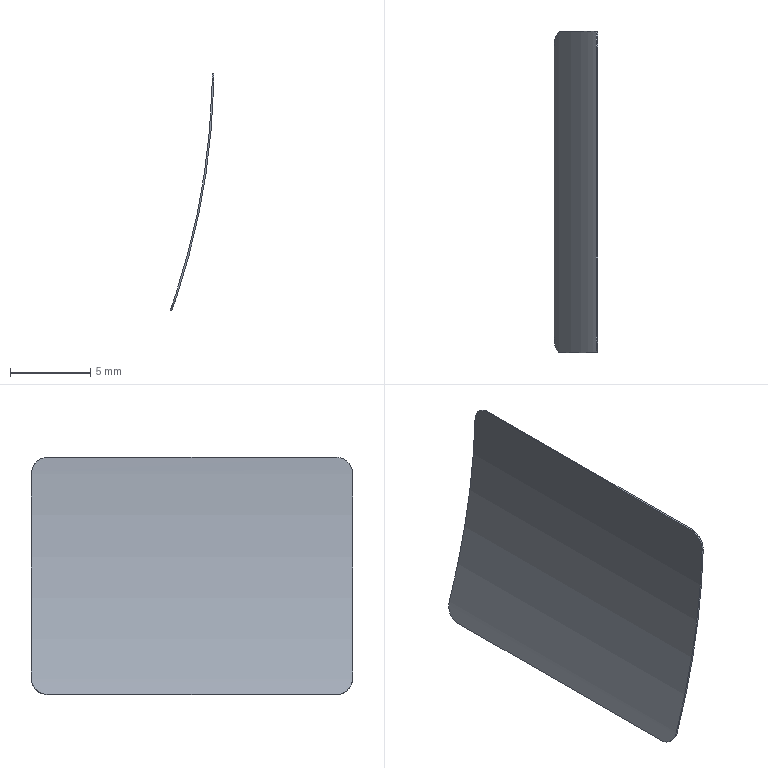Part | SolidWorks | features BaseBody 1 | 1 solid | 10 faces | box 2.721 x 20 x 14.787 mm | volume 30.051 mm3 | cylinder 6 | plane 4 | commonest cylinder face diameters 2 x4 90.8 x1 91 x1
STEP:
#1=CARTESIAN_POINT('',(2075.604,-17.405,824.629));
#2=VERTEX_POINT('',#1);
#3=CARTESIAN_POINT('',(2077.876,-17.405,837.429));
#4=VERTEX_POINT('',#3);
#5=CARTESIAN_POINT('',(2032.4,-17.405,838.898));
#6=DIRECTION('',(0.,-1.,0.));
#7=DIRECTION('',(0.9496,0.,-0.3136));
#8=AXIS2_PLACEMENT_3D('',#5,#6,#7);
#9=CIRCLE('',#8,45.5);
#10=EDGE_CURVE('',#2,#4,#9,.T.);
#11=ORIENTED_EDGE('',*,*,#10,.F.);
#12=CARTESIAN_POINT('',(2075.505,-17.405,824.646));
#13=VERTEX_POINT('',#12);
#14=CARTESIAN_POINT('',(2075.604,-17.405,824.629));
#15=DIRECTION('',(-0.9846,0.,0.1747));
#16=VECTOR('',#15,1000.);
#17=LINE('',#14,#16);
#18=EDGE_CURVE('',#2,#13,#17,.T.);
#19=ORIENTED_EDGE('',*,*,#18,.T.);
#20=CARTESIAN_POINT('',(2077.776,-17.405,837.446));
#21=VERTEX_POINT('',#20);
#22=CARTESIAN_POINT('',(2032.4,-17.405,838.898));
#23=DIRECTION('',(0.,1.,0.));
#24=DIRECTION('',(0.9995,0.,-0.03198));
#25=AXIS2_PLACEMENT_3D('',#22,#23,#24);
#26=CIRCLE('',#25,45.4);
#27=EDGE_CURVE('',#21,#13,#26,.T.);
#28=ORIENTED_EDGE('',*,*,#27,.F.);
#29=CARTESIAN_POINT('',(2077.776,-17.405,837.446));
#30=DIRECTION('',(0.9846,0.,-0.1747));
#31=VECTOR('',#30,1000.);
#32=LINE('',#29,#31);
#33=EDGE_CURVE('',#21,#4,#32,.T.);
#34=ORIENTED_EDGE('',*,*,#33,.T.);
#35=EDGE_LOOP('',(#11,#19,#28,#34));
#36=FACE_OUTER_BOUND('',#35,.T.);
#37=CARTESIAN_POINT('',(2032.4,-17.405,838.898));
#38=DIRECTION('',(0.,-1.,0.));
#39=DIRECTION('',(-0.1747,0.,-0.9846));
#40=AXIS2_PLACEMENT_3D('',#37,#38,#39);
#41=PLANE('',#40);
#42=ADVANCED_FACE('',(#36),#41,.F.);
#43=CARTESIAN_POINT('',(2077.897,-18.405,838.44));
#44=VERTEX_POINT('',#43);
#45=CARTESIAN_POINT('',(2077.876,-17.405,837.429));
#46=CARTESIAN_POINT('',(2077.88,-17.405,837.561));
#47=CARTESIAN_POINT('',(2077.884,-17.431,837.692));
#48=CARTESIAN_POINT('',(2077.89,-17.53,837.936));
#49=CARTESIAN_POINT('',(2077.892,-17.604,838.048));
#50=CARTESIAN_POINT('',(2077.896,-17.88,838.329));
#51=CARTESIAN_POINT('',(2077.897,-18.139,838.44));
#52=CARTESIAN_POINT('',(2077.897,-18.405,838.44));
#53=B_SPLINE_CURVE_WITH_KNOTS('',3,(#45,#46,#47,#48,#49,#50,#51,#52),.UNSPECIFIED.,.F.,.F.,(4,2,2,4),(0.,0.0003928,0.0007857,0.001571),.UNSPECIFIED.);
#54=EDGE_CURVE('',#4,#44,#53,.T.);
#55=ORIENTED_EDGE('',*,*,#54,.F.);
#56=ORIENTED_EDGE('',*,*,#33,.F.);
#57=CARTESIAN_POINT('',(2077.797,-18.405,838.458));
#58=VERTEX_POINT('',#57);
#59=CARTESIAN_POINT('',(2077.797,-18.405,838.458));
#60=CARTESIAN_POINT('',(2077.797,-18.272,838.458));
#61=CARTESIAN_POINT('',(2077.797,-18.142,838.431));
#62=CARTESIAN_POINT('',(2077.796,-17.899,838.329));
#63=CARTESIAN_POINT('',(2077.795,-17.788,838.253));
#64=CARTESIAN_POINT('',(2077.792,-17.604,838.066));
#65=CARTESIAN_POINT('',(2077.79,-17.53,837.953));
#66=CARTESIAN_POINT('',(2077.784,-17.431,837.711));
#67=CARTESIAN_POINT('',(2077.781,-17.405,837.579));
#68=CARTESIAN_POINT('',(2077.776,-17.405,837.446));
#69=B_SPLINE_CURVE_WITH_KNOTS('',3,(#59,#60,#61,#62,#63,#64,#65,#66,#67,#68),.UNSPECIFIED.,.F.,.F.,(4,2,2,2,4),(0.,0.0003929,0.0007857,0.001179,0.001571),.UNSPECIFIED.);
#70=EDGE_CURVE('',#58,#21,#69,.T.);
#71=ORIENTED_EDGE('',*,*,#70,.F.);
#72=CARTESIAN_POINT('',(2077.797,-18.405,838.458));
#73=DIRECTION('',(0.9846,0.,-0.1747));
#74=VECTOR('',#73,1000.);
#75=LINE('',#72,#74);
#76=EDGE_CURVE('',#58,#44,#75,.T.);
#77=ORIENTED_EDGE('',*,*,#76,.T.);
#78=EDGE_LOOP('',(#55,#56,#71,#77));
#79=FACE_OUTER_BOUND('',#78,.T.);
#80=CARTESIAN_POINT('',(2077.583,-18.405,837.481));
#81=DIRECTION('',(0.9846,0.,-0.1747));
#82=DIRECTION('',(0.,-1.,0.));
#83=AXIS2_PLACEMENT_3D('',#80,#81,#82);
#84=CYLINDRICAL_SURFACE('',#83,1.);
#85=ADVANCED_FACE('',(#79),#84,.T.);
#86=CARTESIAN_POINT('',(2077.797,-36.405,838.458));
#87=VERTEX_POINT('',#86);
#88=CARTESIAN_POINT('',(2077.797,-18.405,838.458));
#89=DIRECTION('',(0.,-1.,0.));
#90=VECTOR('',#89,1000.);
#91=LINE('',#88,#90);
#92=EDGE_CURVE('',#58,#87,#91,.T.);
#93=ORIENTED_EDGE('',*,*,#92,.T.);
#94=CARTESIAN_POINT('',(2077.897,-36.405,838.44));
#95=VERTEX_POINT('',#94);
#96=CARTESIAN_POINT('',(2077.897,-36.405,838.44));
#97=DIRECTION('',(-0.9846,0.,0.1747));
#98=VECTOR('',#97,1000.);
#99=LINE('',#96,#98);
#100=EDGE_CURVE('',#95,#87,#99,.T.);
#101=ORIENTED_EDGE('',*,*,#100,.F.);
#102=CARTESIAN_POINT('',(2077.897,-18.405,838.44));
#103=DIRECTION('',(0.,-1.,0.));
#104=VECTOR('',#103,1000.);
#105=LINE('',#102,#104);
#106=EDGE_CURVE('',#44,#95,#105,.T.);
#107=ORIENTED_EDGE('',*,*,#106,.F.);
#108=ORIENTED_EDGE('',*,*,#76,.F.);
#109=EDGE_LOOP('',(#93,#101,#107,#108));
#110=FACE_OUTER_BOUND('',#109,.T.);
#111=CARTESIAN_POINT('',(2077.897,-17.405,838.44));
#112=DIRECTION('',(0.1747,0.,0.9846));
#113=DIRECTION('',(0.9846,0.,-0.1747));
#114=AXIS2_PLACEMENT_3D('',#111,#112,#113);
#115=PLANE('',#114);
#116=ADVANCED_FACE('',(#110),#115,.T.);
#117=ORIENTED_EDGE('',*,*,#106,.T.);
#118=CARTESIAN_POINT('',(2077.876,-37.405,837.429));
#119=VERTEX_POINT('',#118);
#120=CARTESIAN_POINT('',(2077.897,-36.405,838.44));
#121=CARTESIAN_POINT('',(2077.897,-36.538,838.44));
#122=CARTESIAN_POINT('',(2077.897,-36.668,838.414));
#123=CARTESIAN_POINT('',(2077.896,-36.911,838.311));
#124=CARTESIAN_POINT('',(2077.895,-37.022,838.236));
#125=CARTESIAN_POINT('',(2077.892,-37.206,838.049));
#126=CARTESIAN_POINT('',(2077.89,-37.28,837.936));
#127=CARTESIAN_POINT('',(2077.884,-37.379,837.693));
#128=CARTESIAN_POINT('',(2077.88,-37.405,837.561));
#129=CARTESIAN_POINT('',(2077.876,-37.405,837.429));
#130=B_SPLINE_CURVE_WITH_KNOTS('',3,(#120,#121,#122,#123,#124,#125,#126,#127,#128,#129),.UNSPECIFIED.,.F.,.F.,(4,2,2,2,4),(0.,0.0003928,0.0007857,0.001179,0.001571),.UNSPECIFIED.);
#131=EDGE_CURVE('',#95,#119,#130,.T.);
#132=ORIENTED_EDGE('',*,*,#131,.T.);
#133=CARTESIAN_POINT('',(2075.604,-37.405,824.629));
#134=VERTEX_POINT('',#133);
#135=CARTESIAN_POINT('',(2032.4,-37.405,838.898));
#136=DIRECTION('',(0.,-1.,0.));
#137=DIRECTION('',(0.9496,0.,-0.3136));
#138=AXIS2_PLACEMENT_3D('',#135,#136,#137);
#139=CIRCLE('',#138,45.5);
#140=EDGE_CURVE('',#134,#119,#139,.T.);
#141=ORIENTED_EDGE('',*,*,#140,.F.);
#142=CARTESIAN_POINT('',(2075.276,-36.405,823.671));
#143=VERTEX_POINT('',#142);
#144=CARTESIAN_POINT('',(2075.604,-37.405,824.629));
#145=CARTESIAN_POINT('',(2075.562,-37.405,824.503));
#146=CARTESIAN_POINT('',(2075.521,-37.379,824.379));
#147=CARTESIAN_POINT('',(2075.442,-37.28,824.148));
#148=CARTESIAN_POINT('',(2075.406,-37.206,824.042));
#149=CARTESIAN_POINT('',(2075.314,-36.93,823.776));
#150=CARTESIAN_POINT('',(2075.276,-36.671,823.671));
#151=CARTESIAN_POINT('',(2075.276,-36.405,823.671));
#152=B_SPLINE_CURVE_WITH_KNOTS('',3,(#144,#145,#146,#147,#148,#149,#150,#151),.UNSPECIFIED.,.F.,.F.,(4,2,2,4),(0.,0.0003928,0.0007857,0.001571),.UNSPECIFIED.);
#153=EDGE_CURVE('',#134,#143,#152,.T.);
#154=ORIENTED_EDGE('',*,*,#153,.T.);
#155=CARTESIAN_POINT('',(2075.276,-18.405,823.671));
#156=VERTEX_POINT('',#155);
#157=CARTESIAN_POINT('',(2075.276,-18.405,823.671));
#158=DIRECTION('',(0.,-1.,0.));
#159=VECTOR('',#158,1000.);
#160=LINE('',#157,#159);
#161=EDGE_CURVE('',#156,#143,#160,.T.);
#162=ORIENTED_EDGE('',*,*,#161,.F.);
#163=CARTESIAN_POINT('',(2075.276,-18.405,823.671));
#164=CARTESIAN_POINT('',(2075.276,-18.272,823.671));
#165=CARTESIAN_POINT('',(2075.285,-18.142,823.696));
#166=CARTESIAN_POINT('',(2075.319,-17.899,823.793));
#167=CARTESIAN_POINT('',(2075.344,-17.788,823.865));
#168=CARTESIAN_POINT('',(2075.406,-17.604,824.041));
#169=CARTESIAN_POINT('',(2075.442,-17.53,824.148));
#170=CARTESIAN_POINT('',(2075.52,-17.431,824.377));
#171=CARTESIAN_POINT('',(2075.562,-17.405,824.503));
#172=CARTESIAN_POINT('',(2075.604,-17.405,824.629));
#173=B_SPLINE_CURVE_WITH_KNOTS('',3,(#163,#164,#165,#166,#167,#168,#169,#170,#171,#172),.UNSPECIFIED.,.F.,.F.,(4,2,2,2,4),(0.,0.0003928,0.0007857,0.001179,0.001571),.UNSPECIFIED.);
#174=EDGE_CURVE('',#156,#2,#173,.T.);
#175=ORIENTED_EDGE('',*,*,#174,.T.);
#176=ORIENTED_EDGE('',*,*,#10,.T.);
#177=ORIENTED_EDGE('',*,*,#54,.T.);
#178=EDGE_LOOP('',(#117,#132,#141,#154,#162,#175,#176,#177));
#179=FACE_OUTER_BOUND('',#178,.T.);
#180=CARTESIAN_POINT('',(2032.4,-17.405,838.898));
#181=DIRECTION('',(0.,-1.,0.));
#182=DIRECTION('',(-0.1747,0.,-0.9846));
#183=AXIS2_PLACEMENT_3D('',#180,#181,#182);
#184=CYLINDRICAL_SURFACE('',#183,45.5);
#185=ADVANCED_FACE('',(#179),#184,.T.);
#186=CARTESIAN_POINT('',(2075.176,-18.405,823.689));
#187=VERTEX_POINT('',#186);
#188=CARTESIAN_POINT('',(2075.505,-17.405,824.646));
#189=CARTESIAN_POINT('',(2075.463,-17.405,824.52));
#190=CARTESIAN_POINT('',(2075.421,-17.431,824.397));
#191=CARTESIAN_POINT('',(2075.343,-17.53,824.165));
#192=CARTESIAN_POINT('',(2075.306,-17.604,824.06));
#193=CARTESIAN_POINT('',(2075.214,-17.88,823.794));
#194=CARTESIAN_POINT('',(2075.176,-18.139,823.689));
#195=CARTESIAN_POINT('',(2075.176,-18.405,823.689));
#196=B_SPLINE_CURVE_WITH_KNOTS('',3,(#188,#189,#190,#191,#192,#193,#194,#195),.UNSPECIFIED.,.F.,.F.,(4,2,2,4),(0.,0.0003929,0.0007857,0.001571),.UNSPECIFIED.);
#197=EDGE_CURVE('',#13,#187,#196,.T.);
#198=ORIENTED_EDGE('',*,*,#197,.F.);
#199=ORIENTED_EDGE('',*,*,#18,.F.);
#200=ORIENTED_EDGE('',*,*,#174,.F.);
#201=CARTESIAN_POINT('',(2075.276,-18.405,823.671));
#202=DIRECTION('',(-0.9846,0.,0.1747));
#203=VECTOR('',#202,1000.);
#204=LINE('',#201,#203);
#205=EDGE_CURVE('',#156,#187,#204,.T.);
#206=ORIENTED_EDGE('',*,*,#205,.T.);
#207=EDGE_LOOP('',(#198,#199,#200,#206));
#208=FACE_OUTER_BOUND('',#207,.T.);
#209=CARTESIAN_POINT('',(2076.105,-18.405,824.54));
#210=DIRECTION('',(-0.9846,0.,0.1747));
#211=DIRECTION('',(0.,-1.,0.));
#212=AXIS2_PLACEMENT_3D('',#209,#210,#211);
#213=CYLINDRICAL_SURFACE('',#212,1.);
#214=ADVANCED_FACE('',(#208),#213,.T.);
#215=ORIENTED_EDGE('',*,*,#161,.T.);
#216=CARTESIAN_POINT('',(2075.176,-36.405,823.689));
#217=VERTEX_POINT('',#216);
#218=CARTESIAN_POINT('',(2075.176,-36.405,823.689));
#219=DIRECTION('',(0.9846,0.,-0.1747));
#220=VECTOR('',#219,1000.);
#221=LINE('',#218,#220);
#222=EDGE_CURVE('',#217,#143,#221,.T.);
#223=ORIENTED_EDGE('',*,*,#222,.F.);
#224=CARTESIAN_POINT('',(2075.176,-18.405,823.689));
#225=DIRECTION('',(0.,-1.,0.));
#226=VECTOR('',#225,1000.);
#227=LINE('',#224,#226);
#228=EDGE_CURVE('',#187,#217,#227,.T.);
#229=ORIENTED_EDGE('',*,*,#228,.F.);
#230=ORIENTED_EDGE('',*,*,#205,.F.);
#231=EDGE_LOOP('',(#215,#223,#229,#230));
#232=FACE_OUTER_BOUND('',#231,.T.);
#233=CARTESIAN_POINT('',(2075.176,-17.405,823.689));
#234=DIRECTION('',(-0.1747,0.,-0.9846));
#235=DIRECTION('',(-0.9846,0.,0.1747));
#236=AXIS2_PLACEMENT_3D('',#233,#234,#235);
#237=PLANE('',#236);
#238=ADVANCED_FACE('',(#232),#237,.T.);
#239=ORIENTED_EDGE('',*,*,#27,.T.);
#240=ORIENTED_EDGE('',*,*,#197,.T.);
#241=ORIENTED_EDGE('',*,*,#228,.T.);
#242=CARTESIAN_POINT('',(2075.505,-37.405,824.646));
#243=VERTEX_POINT('',#242);
#244=CARTESIAN_POINT('',(2075.176,-36.405,823.689));
#245=CARTESIAN_POINT('',(2075.176,-36.538,823.689));
#246=CARTESIAN_POINT('',(2075.185,-36.668,823.714));
#247=CARTESIAN_POINT('',(2075.219,-36.911,823.811));
#248=CARTESIAN_POINT('',(2075.245,-37.022,823.882));
#249=CARTESIAN_POINT('',(2075.306,-37.206,824.059));
#250=CARTESIAN_POINT('',(2075.343,-37.28,824.166));
#251=CARTESIAN_POINT('',(2075.421,-37.379,824.395));
#252=CARTESIAN_POINT('',(2075.463,-37.405,824.52));
#253=CARTESIAN_POINT('',(2075.505,-37.405,824.646));
#254=B_SPLINE_CURVE_WITH_KNOTS('',3,(#244,#245,#246,#247,#248,#249,#250,#251,#252,#253),.UNSPECIFIED.,.F.,.F.,(4,2,2,2,4),(0.,0.0003929,0.0007857,0.001179,0.001571),.UNSPECIFIED.);
#255=EDGE_CURVE('',#217,#243,#254,.T.);
#256=ORIENTED_EDGE('',*,*,#255,.T.);
#257=CARTESIAN_POINT('',(2077.776,-37.405,837.446));
#258=VERTEX_POINT('',#257);
#259=CARTESIAN_POINT('',(2032.4,-37.405,838.898));
#260=DIRECTION('',(0.,1.,0.));
#261=DIRECTION('',(0.9995,0.,-0.03198));
#262=AXIS2_PLACEMENT_3D('',#259,#260,#261);
#263=CIRCLE('',#262,45.4);
#264=EDGE_CURVE('',#258,#243,#263,.T.);
#265=ORIENTED_EDGE('',*,*,#264,.F.);
#266=CARTESIAN_POINT('',(2077.776,-37.405,837.446));
#267=CARTESIAN_POINT('',(2077.781,-37.405,837.579));
#268=CARTESIAN_POINT('',(2077.784,-37.379,837.709));
#269=CARTESIAN_POINT('',(2077.79,-37.28,837.954));
#270=CARTESIAN_POINT('',(2077.792,-37.206,838.066));
#271=CARTESIAN_POINT('',(2077.797,-36.93,838.347));
#272=CARTESIAN_POINT('',(2077.797,-36.671,838.458));
#273=CARTESIAN_POINT('',(2077.797,-36.405,838.458));
#274=B_SPLINE_CURVE_WITH_KNOTS('',3,(#266,#267,#268,#269,#270,#271,#272,#273),.UNSPECIFIED.,.F.,.F.,(4,2,2,4),(0.,0.0003929,0.0007857,0.001571),.UNSPECIFIED.);
#275=EDGE_CURVE('',#258,#87,#274,.T.);
#276=ORIENTED_EDGE('',*,*,#275,.T.);
#277=ORIENTED_EDGE('',*,*,#92,.F.);
#278=ORIENTED_EDGE('',*,*,#70,.T.);
#279=EDGE_LOOP('',(#239,#240,#241,#256,#265,#276,#277,#278));
#280=FACE_OUTER_BOUND('',#279,.T.);
#281=CARTESIAN_POINT('',(2032.4,-17.405,838.898));
#282=DIRECTION('',(0.,-1.,0.));
#283=DIRECTION('',(-0.1747,0.,-0.9846));
#284=AXIS2_PLACEMENT_3D('',#281,#282,#283);
#285=CYLINDRICAL_SURFACE('',#284,45.4);
#286=ADVANCED_FACE('',(#280),#285,.F.);
#287=ORIENTED_EDGE('',*,*,#275,.F.);
#288=CARTESIAN_POINT('',(2077.876,-37.405,837.429));
#289=DIRECTION('',(-0.9846,0.,0.1747));
#290=VECTOR('',#289,1000.);
#291=LINE('',#288,#290);
#292=EDGE_CURVE('',#119,#258,#291,.T.);
#293=ORIENTED_EDGE('',*,*,#292,.F.);
#294=ORIENTED_EDGE('',*,*,#131,.F.);
#295=ORIENTED_EDGE('',*,*,#100,.T.);
#296=EDGE_LOOP('',(#287,#293,#294,#295));
#297=FACE_OUTER_BOUND('',#296,.T.);
#298=CARTESIAN_POINT('',(2078.377,-36.405,837.34));
#299=DIRECTION('',(-0.9846,0.,0.1747));
#300=DIRECTION('',(0.,1.,0.));
#301=AXIS2_PLACEMENT_3D('',#298,#299,#300);
#302=CYLINDRICAL_SURFACE('',#301,1.);
#303=ADVANCED_FACE('',(#297),#302,.T.);
#304=ORIENTED_EDGE('',*,*,#264,.T.);
#305=CARTESIAN_POINT('',(2075.505,-37.405,824.646));
#306=DIRECTION('',(0.9846,0.,-0.1747));
#307=VECTOR('',#306,1000.);
#308=LINE('',#305,#307);
#309=EDGE_CURVE('',#243,#134,#308,.T.);
#310=ORIENTED_EDGE('',*,*,#309,.T.);
#311=ORIENTED_EDGE('',*,*,#140,.T.);
#312=ORIENTED_EDGE('',*,*,#292,.T.);
#313=EDGE_LOOP('',(#304,#310,#311,#312));
#314=FACE_OUTER_BOUND('',#313,.T.);
#315=CARTESIAN_POINT('',(2032.4,-37.405,838.898));
#316=DIRECTION('',(0.,-1.,0.));
#317=DIRECTION('',(-0.1747,0.,-0.9846));
#318=AXIS2_PLACEMENT_3D('',#315,#316,#317);
#319=PLANE('',#318);
#320=ADVANCED_FACE('',(#314),#319,.T.);
#321=ORIENTED_EDGE('',*,*,#153,.F.);
#322=ORIENTED_EDGE('',*,*,#309,.F.);
#323=ORIENTED_EDGE('',*,*,#255,.F.);
#324=ORIENTED_EDGE('',*,*,#222,.T.);
#325=EDGE_LOOP('',(#321,#322,#323,#324));
#326=FACE_OUTER_BOUND('',#325,.T.);
#327=CARTESIAN_POINT('',(2075.311,-36.405,824.681));
#328=DIRECTION('',(0.9846,0.,-0.1747));
#329=DIRECTION('',(0.,1.,0.));
#330=AXIS2_PLACEMENT_3D('',#327,#328,#329);
#331=CYLINDRICAL_SURFACE('',#330,1.);
#332=ADVANCED_FACE('',(#326),#331,.T.);
#333=CLOSED_SHELL('',(#42,#85,#116,#185,#214,#238,#286,#303,#320,#332));
#334=MANIFOLD_SOLID_BREP('',#333);
#335=CARTESIAN_POINT('',(0.,0.,0.));
#336=DIRECTION('',(0.,0.,1.));
#337=DIRECTION('',(1.,0.,0.));
#338=AXIS2_PLACEMENT_3D('',#335,#336,#337);
#339=(LENGTH_UNIT()NAMED_UNIT(*)SI_UNIT(.MILLI.,.METRE.));
#340=UNCERTAINTY_MEASURE_WITH_UNIT(LENGTH_MEASURE(0.00001),#339,'','');
#341=(NAMED_UNIT(*)PLANE_ANGLE_UNIT()SI_UNIT($,.RADIAN.));
#342=(NAMED_UNIT(*)SI_UNIT($,.STERADIAN.)SOLID_ANGLE_UNIT());
#343=(GEOMETRIC_REPRESENTATION_CONTEXT(3)GLOBAL_UNCERTAINTY_ASSIGNED_CONTEXT((#340))GLOBAL_UNIT_ASSIGNED_CONTEXT((#339,#341,#342))REPRESENTATION_CONTEXT('',''));
#344=ADVANCED_BREP_SHAPE_REPRESENTATION('',(#334,#338),#343);